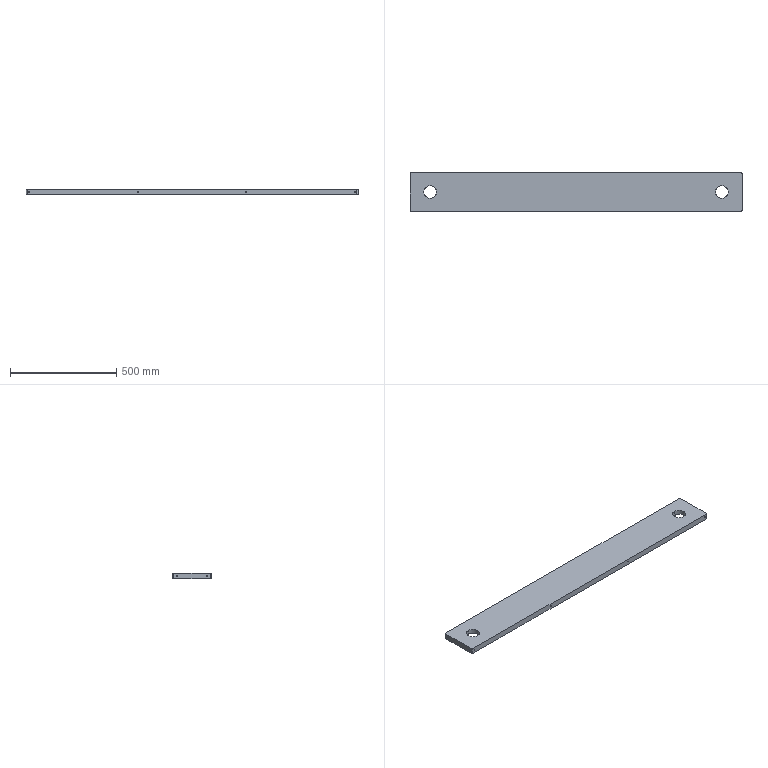Part | SolidWorks | features BaseBody 1 | 1 solid | 92 faces | box 1560 x 180 x 28 mm | volume 7667236 mm3 | cylinder 44 | cone 40 | plane 8 | commonest cylinder face diameters 5 x24 10.2 x8 10 x4 60 x4 80 x4